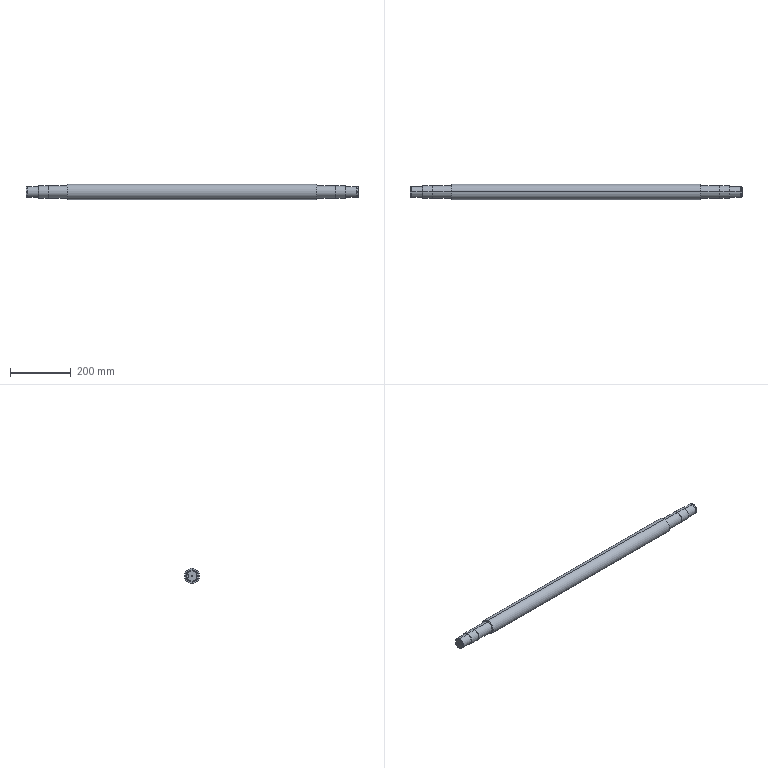Part | SolidWorks | features BaseBody 1 | 1 solid | 72 faces | box 1090 x 50 x 50 mm | volume 1919950 mm3 | cylinder 34 | plane 20 | cone 18 | commonest cylinder face diameters 35 x12 40 x8 33 x6 37 x4 10 x2 50 x2